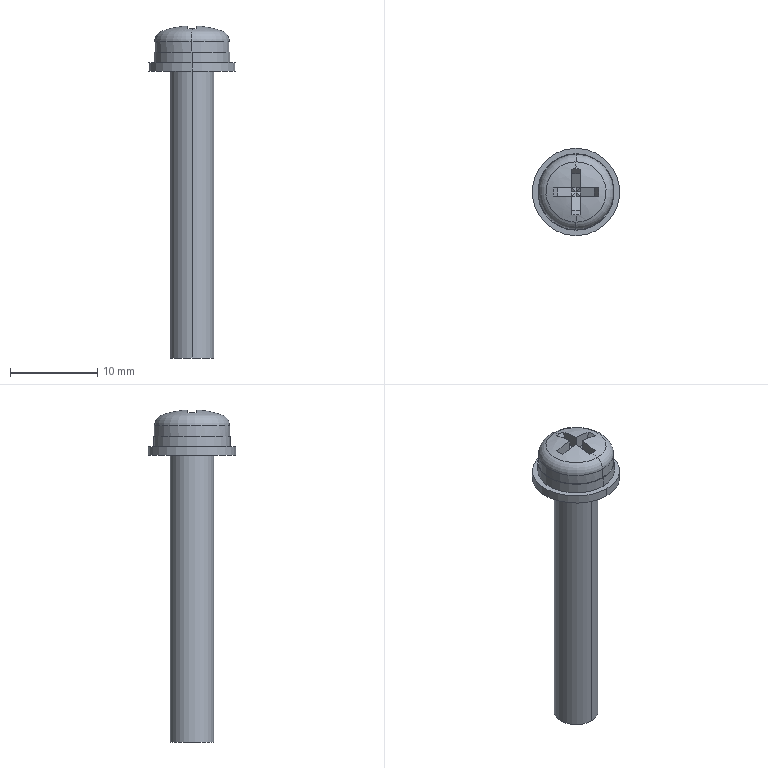Part | STEP file | 1 solid | 44 faces | box 10 x 10 x 37.975 mm | volume 923.659 mm3 | plane 32 | cylinder 8 | torus 2 | sphere 2 | commonest cylinder face diameters 5 x2 8.6 x2 8.75 x2 10 x2